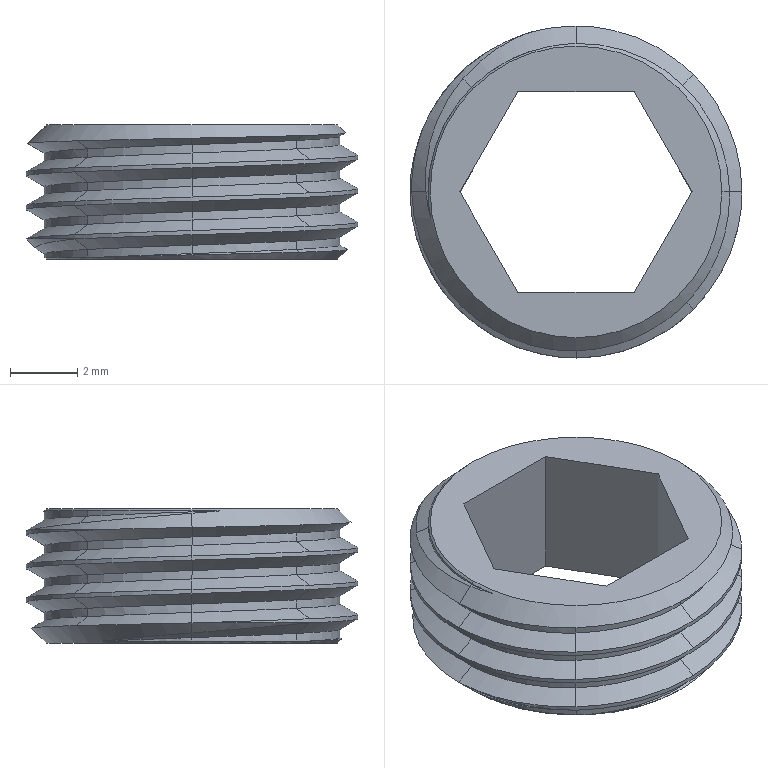Part | NX | features BREP 1 | 1 solid | 118 faces | box 9.9 x 9.9 x 4 mm | volume 143.224 mm3 | spline 64 | cylinder 40 | plane 8 | cone 6 | commonest cylinder face diameters 8.817 x34 9.9 x6